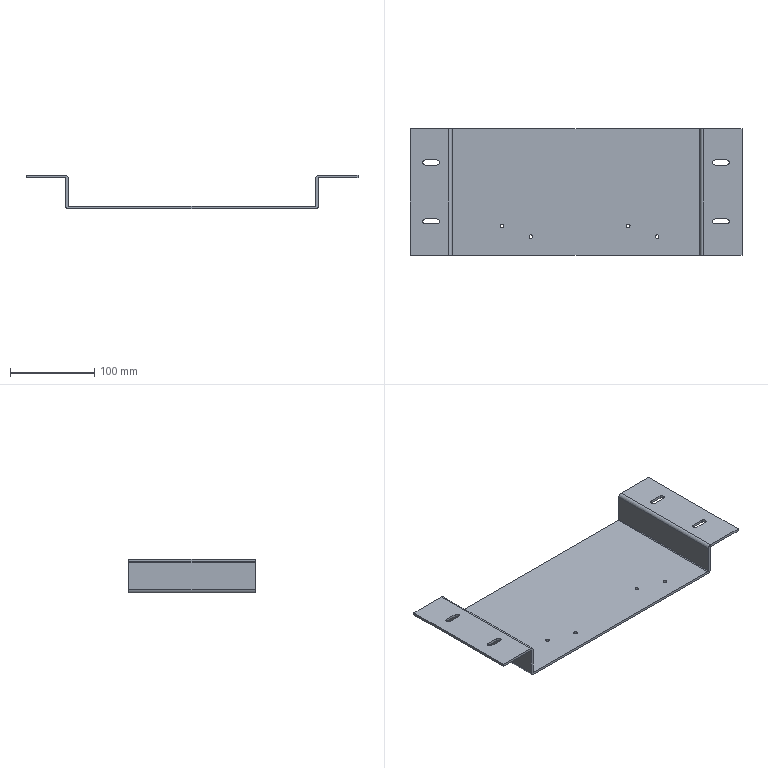Part | SolidWorks | features BaseBody 1 | 1 solid | 46 faces | box 394 x 150 x 40 mm | volume 207359 mm3 | cylinder 24 | plane 22 | commonest cylinder face diameters 4.2 x8 6 x8 1.473 x4 7.473 x4
STEP:
#1=CARTESIAN_POINT('',(98.5,-52.95,0.));
#2=VERTEX_POINT('',#1);
#3=CARTESIAN_POINT('',(94.3,-52.95,0.));
#4=VERTEX_POINT('',#3);
#5=CARTESIAN_POINT('',(96.4,-52.95,0.));
#6=DIRECTION('',(0.,0.,-1.));
#7=DIRECTION('',(-1.,0.,0.));
#8=AXIS2_PLACEMENT_3D('',#5,#6,#7);
#9=CIRCLE('',#8,2.1);
#10=EDGE_CURVE('',#2,#4,#9,.T.);
#11=ORIENTED_EDGE('',*,*,#10,.F.);
#12=CARTESIAN_POINT('',(98.5,-52.95,-3.));
#13=VERTEX_POINT('',#12);
#14=CARTESIAN_POINT('',(98.5,-52.95,-3.));
#15=DIRECTION('',(0.,0.,-1.));
#16=VECTOR('',#15,1000.);
#17=LINE('',#14,#16);
#18=EDGE_CURVE('',#2,#13,#17,.T.);
#19=ORIENTED_EDGE('',*,*,#18,.T.);
#20=CARTESIAN_POINT('',(94.3,-52.95,-3.));
#21=VERTEX_POINT('',#20);
#22=CARTESIAN_POINT('',(96.4,-52.95,-3.));
#23=DIRECTION('',(0.,0.,-1.));
#24=DIRECTION('',(-1.,0.,0.));
#25=AXIS2_PLACEMENT_3D('',#22,#23,#24);
#26=CIRCLE('',#25,2.1);
#27=EDGE_CURVE('',#13,#21,#26,.T.);
#28=ORIENTED_EDGE('',*,*,#27,.T.);
#29=CARTESIAN_POINT('',(94.3,-52.95,-3.));
#30=DIRECTION('',(0.,0.,-1.));
#31=VECTOR('',#30,1000.);
#32=LINE('',#29,#31);
#33=EDGE_CURVE('',#4,#21,#32,.T.);
#34=ORIENTED_EDGE('',*,*,#33,.F.);
#35=EDGE_LOOP('',(#11,#19,#28,#34));
#36=FACE_OUTER_BOUND('',#35,.T.);
#37=CARTESIAN_POINT('',(96.4,-52.95,-3.));
#38=DIRECTION('',(0.,0.,-1.));
#39=DIRECTION('',(-1.,0.,0.));
#40=AXIS2_PLACEMENT_3D('',#37,#38,#39);
#41=CYLINDRICAL_SURFACE('',#40,2.1);
#42=ADVANCED_FACE('',(#36),#41,.F.);
#43=CARTESIAN_POINT('',(64.1,-40.25,0.));
#44=VERTEX_POINT('',#43);
#45=CARTESIAN_POINT('',(59.9,-40.25,0.));
#46=VERTEX_POINT('',#45);
#47=CARTESIAN_POINT('',(62.,-40.25,0.));
#48=DIRECTION('',(0.,0.,-1.));
#49=DIRECTION('',(-1.,0.,0.));
#50=AXIS2_PLACEMENT_3D('',#47,#48,#49);
#51=CIRCLE('',#50,2.1);
#52=EDGE_CURVE('',#44,#46,#51,.T.);
#53=ORIENTED_EDGE('',*,*,#52,.F.);
#54=CARTESIAN_POINT('',(64.1,-40.25,-3.));
#55=VERTEX_POINT('',#54);
#56=CARTESIAN_POINT('',(64.1,-40.25,-3.));
#57=DIRECTION('',(0.,0.,-1.));
#58=VECTOR('',#57,1000.);
#59=LINE('',#56,#58);
#60=EDGE_CURVE('',#44,#55,#59,.T.);
#61=ORIENTED_EDGE('',*,*,#60,.T.);
#62=CARTESIAN_POINT('',(59.9,-40.25,-3.));
#63=VERTEX_POINT('',#62);
#64=CARTESIAN_POINT('',(62.,-40.25,-3.));
#65=DIRECTION('',(0.,0.,-1.));
#66=DIRECTION('',(-1.,0.,0.));
#67=AXIS2_PLACEMENT_3D('',#64,#65,#66);
#68=CIRCLE('',#67,2.1);
#69=EDGE_CURVE('',#55,#63,#68,.T.);
#70=ORIENTED_EDGE('',*,*,#69,.T.);
#71=CARTESIAN_POINT('',(59.9,-40.25,-3.));
#72=DIRECTION('',(0.,0.,-1.));
#73=VECTOR('',#72,1000.);
#74=LINE('',#71,#73);
#75=EDGE_CURVE('',#46,#63,#74,.T.);
#76=ORIENTED_EDGE('',*,*,#75,.F.);
#77=EDGE_LOOP('',(#53,#61,#70,#76));
#78=FACE_OUTER_BOUND('',#77,.T.);
#79=CARTESIAN_POINT('',(62.,-40.25,-3.));
#80=DIRECTION('',(0.,0.,-1.));
#81=DIRECTION('',(-1.,0.,0.));
#82=AXIS2_PLACEMENT_3D('',#79,#80,#81);
#83=CYLINDRICAL_SURFACE('',#82,2.1);
#84=ADVANCED_FACE('',(#78),#83,.F.);
#85=CARTESIAN_POINT('',(-51.5,-52.95,0.));
#86=VERTEX_POINT('',#85);
#87=CARTESIAN_POINT('',(-55.7,-52.95,0.));
#88=VERTEX_POINT('',#87);
#89=CARTESIAN_POINT('',(-53.6,-52.95,0.));
#90=DIRECTION('',(0.,0.,-1.));
#91=DIRECTION('',(-1.,0.,0.));
#92=AXIS2_PLACEMENT_3D('',#89,#90,#91);
#93=CIRCLE('',#92,2.1);
#94=EDGE_CURVE('',#86,#88,#93,.T.);
#95=ORIENTED_EDGE('',*,*,#94,.F.);
#96=CARTESIAN_POINT('',(-51.5,-52.95,-3.));
#97=VERTEX_POINT('',#96);
#98=CARTESIAN_POINT('',(-51.5,-52.95,-3.));
#99=DIRECTION('',(0.,0.,-1.));
#100=VECTOR('',#99,1000.);
#101=LINE('',#98,#100);
#102=EDGE_CURVE('',#86,#97,#101,.T.);
#103=ORIENTED_EDGE('',*,*,#102,.T.);
#104=CARTESIAN_POINT('',(-55.7,-52.95,-3.));
#105=VERTEX_POINT('',#104);
#106=CARTESIAN_POINT('',(-53.6,-52.95,-3.));
#107=DIRECTION('',(0.,0.,-1.));
#108=DIRECTION('',(-1.,0.,0.));
#109=AXIS2_PLACEMENT_3D('',#106,#107,#108);
#110=CIRCLE('',#109,2.1);
#111=EDGE_CURVE('',#97,#105,#110,.T.);
#112=ORIENTED_EDGE('',*,*,#111,.T.);
#113=CARTESIAN_POINT('',(-55.7,-52.95,-3.));
#114=DIRECTION('',(0.,0.,-1.));
#115=VECTOR('',#114,1000.);
#116=LINE('',#113,#115);
#117=EDGE_CURVE('',#88,#105,#116,.T.);
#118=ORIENTED_EDGE('',*,*,#117,.F.);
#119=EDGE_LOOP('',(#95,#103,#112,#118));
#120=FACE_OUTER_BOUND('',#119,.T.);
#121=CARTESIAN_POINT('',(-53.6,-52.95,-3.));
#122=DIRECTION('',(0.,0.,-1.));
#123=DIRECTION('',(-1.,0.,0.));
#124=AXIS2_PLACEMENT_3D('',#121,#122,#123);
#125=CYLINDRICAL_SURFACE('',#124,2.1);
#126=ADVANCED_FACE('',(#120),#125,.F.);
#127=CARTESIAN_POINT('',(-85.9,-40.25,0.));
#128=VERTEX_POINT('',#127);
#129=CARTESIAN_POINT('',(-90.1,-40.25,0.));
#130=VERTEX_POINT('',#129);
#131=CARTESIAN_POINT('',(-88.,-40.25,0.));
#132=DIRECTION('',(0.,0.,-1.));
#133=DIRECTION('',(-1.,0.,0.));
#134=AXIS2_PLACEMENT_3D('',#131,#132,#133);
#135=CIRCLE('',#134,2.1);
#136=EDGE_CURVE('',#128,#130,#135,.T.);
#137=ORIENTED_EDGE('',*,*,#136,.F.);
#138=CARTESIAN_POINT('',(-85.9,-40.25,-3.));
#139=VERTEX_POINT('',#138);
#140=CARTESIAN_POINT('',(-85.9,-40.25,-3.));
#141=DIRECTION('',(0.,0.,-1.));
#142=VECTOR('',#141,1000.);
#143=LINE('',#140,#142);
#144=EDGE_CURVE('',#128,#139,#143,.T.);
#145=ORIENTED_EDGE('',*,*,#144,.T.);
#146=CARTESIAN_POINT('',(-90.1,-40.25,-3.));
#147=VERTEX_POINT('',#146);
#148=CARTESIAN_POINT('',(-88.,-40.25,-3.));
#149=DIRECTION('',(0.,0.,-1.));
#150=DIRECTION('',(-1.,0.,0.));
#151=AXIS2_PLACEMENT_3D('',#148,#149,#150);
#152=CIRCLE('',#151,2.1);
#153=EDGE_CURVE('',#139,#147,#152,.T.);
#154=ORIENTED_EDGE('',*,*,#153,.T.);
#155=CARTESIAN_POINT('',(-90.1,-40.25,-3.));
#156=DIRECTION('',(0.,0.,-1.));
#157=VECTOR('',#156,1000.);
#158=LINE('',#155,#157);
#159=EDGE_CURVE('',#130,#147,#158,.T.);
#160=ORIENTED_EDGE('',*,*,#159,.F.);
#161=EDGE_LOOP('',(#137,#145,#154,#160));
#162=FACE_OUTER_BOUND('',#161,.T.);
#163=CARTESIAN_POINT('',(-88.,-40.25,-3.));
#164=DIRECTION('',(0.,0.,-1.));
#165=DIRECTION('',(-1.,0.,0.));
#166=AXIS2_PLACEMENT_3D('',#163,#164,#165);
#167=CYLINDRICAL_SURFACE('',#166,2.1);
#168=ADVANCED_FACE('',(#162),#167,.F.);
#169=CARTESIAN_POINT('',(165.,32.,34.));
#170=VERTEX_POINT('',#169);
#171=CARTESIAN_POINT('',(165.,32.,37.));
#172=VERTEX_POINT('',#171);
#173=CARTESIAN_POINT('',(165.,32.,34.));
#174=DIRECTION('',(0.,0.,1.));
#175=VECTOR('',#174,1000.);
#176=LINE('',#173,#175);
#177=EDGE_CURVE('',#170,#172,#176,.T.);
#178=ORIENTED_EDGE('',*,*,#177,.T.);
#179=CARTESIAN_POINT('',(179.,32.,37.));
#180=VERTEX_POINT('',#179);
#181=CARTESIAN_POINT('',(179.,32.,37.));
#182=DIRECTION('',(-1.,0.,0.));
#183=VECTOR('',#182,1000.);
#184=LINE('',#181,#183);
#185=EDGE_CURVE('',#180,#172,#184,.T.);
#186=ORIENTED_EDGE('',*,*,#185,.F.);
#187=CARTESIAN_POINT('',(179.,32.,34.));
#188=VERTEX_POINT('',#187);
#189=CARTESIAN_POINT('',(179.,32.,34.));
#190=DIRECTION('',(0.,0.,-1.));
#191=VECTOR('',#190,1000.);
#192=LINE('',#189,#191);
#193=EDGE_CURVE('',#180,#188,#192,.T.);
#194=ORIENTED_EDGE('',*,*,#193,.T.);
#195=CARTESIAN_POINT('',(179.,32.,34.));
#196=DIRECTION('',(-1.,0.,0.));
#197=VECTOR('',#196,1000.);
#198=LINE('',#195,#197);
#199=EDGE_CURVE('',#188,#170,#198,.T.);
#200=ORIENTED_EDGE('',*,*,#199,.T.);
#201=EDGE_LOOP('',(#178,#186,#194,#200));
#202=FACE_OUTER_BOUND('',#201,.T.);
#203=CARTESIAN_POINT('',(179.,32.,34.));
#204=DIRECTION('',(0.,-1.,0.));
#205=DIRECTION('',(-1.,0.,0.));
#206=AXIS2_PLACEMENT_3D('',#203,#204,#205);
#207=PLANE('',#206);
#208=ADVANCED_FACE('',(#202),#207,.F.);
#209=CARTESIAN_POINT('',(165.,38.,37.));
#210=VERTEX_POINT('',#209);
#211=CARTESIAN_POINT('',(165.,38.,34.));
#212=VERTEX_POINT('',#211);
#213=CARTESIAN_POINT('',(165.,38.,34.));
#214=DIRECTION('',(0.,0.,-1.));
#215=VECTOR('',#214,1000.);
#216=LINE('',#213,#215);
#217=EDGE_CURVE('',#210,#212,#216,.T.);
#218=ORIENTED_EDGE('',*,*,#217,.T.);
#219=CARTESIAN_POINT('',(179.,38.,34.));
#220=VERTEX_POINT('',#219);
#221=CARTESIAN_POINT('',(179.,38.,34.));
#222=DIRECTION('',(-1.,0.,0.));
#223=VECTOR('',#222,1000.);
#224=LINE('',#221,#223);
#225=EDGE_CURVE('',#220,#212,#224,.T.);
#226=ORIENTED_EDGE('',*,*,#225,.F.);
#227=CARTESIAN_POINT('',(179.,38.,37.));
#228=VERTEX_POINT('',#227);
#229=CARTESIAN_POINT('',(179.,38.,34.));
#230=DIRECTION('',(0.,0.,1.));
#231=VECTOR('',#230,1000.);
#232=LINE('',#229,#231);
#233=EDGE_CURVE('',#220,#228,#232,.T.);
#234=ORIENTED_EDGE('',*,*,#233,.T.);
#235=CARTESIAN_POINT('',(179.,38.,37.));
#236=DIRECTION('',(-1.,0.,0.));
#237=VECTOR('',#236,1000.);
#238=LINE('',#235,#237);
#239=EDGE_CURVE('',#228,#210,#238,.T.);
#240=ORIENTED_EDGE('',*,*,#239,.T.);
#241=EDGE_LOOP('',(#218,#226,#234,#240));
#242=FACE_OUTER_BOUND('',#241,.T.);
#243=CARTESIAN_POINT('',(179.,38.,34.));
#244=DIRECTION('',(0.,1.,0.));
#245=DIRECTION('',(0.,0.,-1.));
#246=AXIS2_PLACEMENT_3D('',#243,#244,#245);
#247=PLANE('',#246);
#248=ADVANCED_FACE('',(#242),#247,.F.);
#249=CARTESIAN_POINT('',(179.,35.,34.));
#250=DIRECTION('',(0.,0.,-1.));
#251=DIRECTION('',(0.,1.,0.));
#252=AXIS2_PLACEMENT_3D('',#249,#250,#251);
#253=CIRCLE('',#252,3.);
#254=EDGE_CURVE('',#220,#188,#253,.T.);
#255=ORIENTED_EDGE('',*,*,#254,.T.);
#256=ORIENTED_EDGE('',*,*,#193,.F.);
#257=CARTESIAN_POINT('',(179.,35.,37.));
#258=DIRECTION('',(0.,0.,-1.));
#259=DIRECTION('',(0.,1.,0.));
#260=AXIS2_PLACEMENT_3D('',#257,#258,#259);
#261=CIRCLE('',#260,3.);
#262=EDGE_CURVE('',#228,#180,#261,.T.);
#263=ORIENTED_EDGE('',*,*,#262,.F.);
#264=ORIENTED_EDGE('',*,*,#233,.F.);
#265=EDGE_LOOP('',(#255,#256,#263,#264));
#266=FACE_OUTER_BOUND('',#265,.T.);
#267=CARTESIAN_POINT('',(179.,35.,34.));
#268=DIRECTION('',(0.,0.,-1.));
#269=DIRECTION('',(0.,1.,0.));
#270=AXIS2_PLACEMENT_3D('',#267,#268,#269);
#271=CYLINDRICAL_SURFACE('',#270,3.);
#272=ADVANCED_FACE('',(#266),#271,.F.);
#273=CARTESIAN_POINT('',(165.,35.,34.));
#274=DIRECTION('',(0.,0.,-1.));
#275=DIRECTION('',(0.,1.,0.));
#276=AXIS2_PLACEMENT_3D('',#273,#274,#275);
#277=CIRCLE('',#276,3.);
#278=EDGE_CURVE('',#170,#212,#277,.T.);
#279=ORIENTED_EDGE('',*,*,#278,.T.);
#280=ORIENTED_EDGE('',*,*,#217,.F.);
#281=CARTESIAN_POINT('',(165.,35.,37.));
#282=DIRECTION('',(0.,0.,-1.));
#283=DIRECTION('',(0.,1.,0.));
#284=AXIS2_PLACEMENT_3D('',#281,#282,#283);
#285=CIRCLE('',#284,3.);
#286=EDGE_CURVE('',#172,#210,#285,.T.);
#287=ORIENTED_EDGE('',*,*,#286,.F.);
#288=ORIENTED_EDGE('',*,*,#177,.F.);
#289=EDGE_LOOP('',(#279,#280,#287,#288));
#290=FACE_OUTER_BOUND('',#289,.T.);
#291=CARTESIAN_POINT('',(165.,35.,34.));
#292=DIRECTION('',(0.,0.,-1.));
#293=DIRECTION('',(0.,1.,0.));
#294=AXIS2_PLACEMENT_3D('',#291,#292,#293);
#295=CYLINDRICAL_SURFACE('',#294,3.);
#296=ADVANCED_FACE('',(#290),#295,.F.);
#297=CARTESIAN_POINT('',(165.,-38.,34.));
#298=VERTEX_POINT('',#297);
#299=CARTESIAN_POINT('',(165.,-38.,37.));
#300=VERTEX_POINT('',#299);
#301=CARTESIAN_POINT('',(165.,-38.,34.));
#302=DIRECTION('',(0.,0.,1.));
#303=VECTOR('',#302,1000.);
#304=LINE('',#301,#303);
#305=EDGE_CURVE('',#298,#300,#304,.T.);
#306=ORIENTED_EDGE('',*,*,#305,.T.);
#307=CARTESIAN_POINT('',(179.,-38.,37.));
#308=VERTEX_POINT('',#307);
#309=CARTESIAN_POINT('',(179.,-38.,37.));
#310=DIRECTION('',(-1.,0.,0.));
#311=VECTOR('',#310,1000.);
#312=LINE('',#309,#311);
#313=EDGE_CURVE('',#308,#300,#312,.T.);
#314=ORIENTED_EDGE('',*,*,#313,.F.);
#315=CARTESIAN_POINT('',(179.,-38.,34.));
#316=VERTEX_POINT('',#315);
#317=CARTESIAN_POINT('',(179.,-38.,34.));
#318=DIRECTION('',(0.,0.,-1.));
#319=VECTOR('',#318,1000.);
#320=LINE('',#317,#319);
#321=EDGE_CURVE('',#308,#316,#320,.T.);
#322=ORIENTED_EDGE('',*,*,#321,.T.);
#323=CARTESIAN_POINT('',(179.,-38.,34.));
#324=DIRECTION('',(-1.,0.,0.));
#325=VECTOR('',#324,1000.);
#326=LINE('',#323,#325);
#327=EDGE_CURVE('',#316,#298,#326,.T.);
#328=ORIENTED_EDGE('',*,*,#327,.T.);
#329=EDGE_LOOP('',(#306,#314,#322,#328));
#330=FACE_OUTER_BOUND('',#329,.T.);
#331=CARTESIAN_POINT('',(179.,-38.,34.));
#332=DIRECTION('',(0.,-1.,0.));
#333=DIRECTION('',(-1.,0.,0.));
#334=AXIS2_PLACEMENT_3D('',#331,#332,#333);
#335=PLANE('',#334);
#336=ADVANCED_FACE('',(#330),#335,.F.);
#337=CARTESIAN_POINT('',(165.,-32.,37.));
#338=VERTEX_POINT('',#337);
#339=CARTESIAN_POINT('',(165.,-32.,34.));
#340=VERTEX_POINT('',#339);
#341=CARTESIAN_POINT('',(165.,-32.,34.));
#342=DIRECTION('',(0.,0.,-1.));
#343=VECTOR('',#342,1000.);
#344=LINE('',#341,#343);
#345=EDGE_CURVE('',#338,#340,#344,.T.);
#346=ORIENTED_EDGE('',*,*,#345,.T.);
#347=CARTESIAN_POINT('',(179.,-32.,34.));
#348=VERTEX_POINT('',#347);
#349=CARTESIAN_POINT('',(179.,-32.,34.));
#350=DIRECTION('',(-1.,0.,0.));
#351=VECTOR('',#350,1000.);
#352=LINE('',#349,#351);
#353=EDGE_CURVE('',#348,#340,#352,.T.);
#354=ORIENTED_EDGE('',*,*,#353,.F.);
#355=CARTESIAN_POINT('',(179.,-32.,37.));
#356=VERTEX_POINT('',#355);
#357=CARTESIAN_POINT('',(179.,-32.,34.));
#358=DIRECTION('',(0.,0.,1.));
#359=VECTOR('',#358,1000.);
#360=LINE('',#357,#359);
#361=EDGE_CURVE('',#348,#356,#360,.T.);
#362=ORIENTED_EDGE('',*,*,#361,.T.);
#363=CARTESIAN_POINT('',(179.,-32.,37.));
#364=DIRECTION('',(-1.,0.,0.));
#365=VECTOR('',#364,1000.);
#366=LINE('',#363,#365);
#367=EDGE_CURVE('',#356,#338,#366,.T.);
#368=ORIENTED_EDGE('',*,*,#367,.T.);
#369=EDGE_LOOP('',(#346,#354,#362,#368));
#370=FACE_OUTER_BOUND('',#369,.T.);
#371=CARTESIAN_POINT('',(179.,-32.,34.));
#372=DIRECTION('',(0.,1.,0.));
#373=DIRECTION('',(0.,0.,-1.));
#374=AXIS2_PLACEMENT_3D('',#371,#372,#373);
#375=PLANE('',#374);
#376=ADVANCED_FACE('',(#370),#375,.F.);
#377=CARTESIAN_POINT('',(179.,-35.,34.));
#378=DIRECTION('',(0.,0.,-1.));
#379=DIRECTION('',(0.,1.,0.));
#380=AXIS2_PLACEMENT_3D('',#377,#378,#379);
#381=CIRCLE('',#380,3.);
#382=EDGE_CURVE('',#348,#316,#381,.T.);
#383=ORIENTED_EDGE('',*,*,#382,.T.);
#384=ORIENTED_EDGE('',*,*,#321,.F.);
#385=CARTESIAN_POINT('',(179.,-35.,37.));
#386=DIRECTION('',(0.,0.,-1.));
#387=DIRECTION('',(0.,1.,0.));
#388=AXIS2_PLACEMENT_3D('',#385,#386,#387);
#389=CIRCLE('',#388,3.);
#390=EDGE_CURVE('',#356,#308,#389,.T.);
#391=ORIENTED_EDGE('',*,*,#390,.F.);
#392=ORIENTED_EDGE('',*,*,#361,.F.);
#393=EDGE_LOOP('',(#383,#384,#391,#392));
#394=FACE_OUTER_BOUND('',#393,.T.);
#395=CARTESIAN_POINT('',(179.,-35.,34.));
#396=DIRECTION('',(0.,0.,-1.));
#397=DIRECTION('',(0.,1.,0.));
#398=AXIS2_PLACEMENT_3D('',#395,#396,#397);
#399=CYLINDRICAL_SURFACE('',#398,3.);
#400=ADVANCED_FACE('',(#394),#399,.F.);
#401=CARTESIAN_POINT('',(165.,-35.,34.));
#402=DIRECTION('',(0.,0.,-1.));
#403=DIRECTION('',(0.,1.,0.));
#404=AXIS2_PLACEMENT_3D('',#401,#402,#403);
#405=CIRCLE('',#404,3.);
#406=EDGE_CURVE('',#298,#340,#405,.T.);
#407=ORIENTED_EDGE('',*,*,#406,.T.);
#408=ORIENTED_EDGE('',*,*,#345,.F.);
#409=CARTESIAN_POINT('',(165.,-35.,37.));
#410=DIRECTION('',(0.,0.,-1.));
#411=DIRECTION('',(0.,1.,0.));
#412=AXIS2_PLACEMENT_3D('',#409,#410,#411);
#413=CIRCLE('',#412,3.);
#414=EDGE_CURVE('',#300,#338,#413,.T.);
#415=ORIENTED_EDGE('',*,*,#414,.F.);
#416=ORIENTED_EDGE('',*,*,#305,.F.);
#417=EDGE_LOOP('',(#407,#408,#415,#416));
#418=FACE_OUTER_BOUND('',#417,.T.);
#419=CARTESIAN_POINT('',(165.,-35.,34.));
#420=DIRECTION('',(0.,0.,-1.));
#421=DIRECTION('',(0.,1.,0.));
#422=AXIS2_PLACEMENT_3D('',#419,#420,#421);
#423=CYLINDRICAL_SURFACE('',#422,3.);
#424=ADVANCED_FACE('',(#418),#423,.F.);
#425=CARTESIAN_POINT('',(-179.,-38.,34.));
#426=VERTEX_POINT('',#425);
#427=CARTESIAN_POINT('',(-179.,-38.,37.));
#428=VERTEX_POINT('',#427);
#429=CARTESIAN_POINT('',(-179.,-38.,34.));
#430=DIRECTION('',(0.,0.,1.));
#431=VECTOR('',#430,1000.);
#432=LINE('',#429,#431);
#433=EDGE_CURVE('',#426,#428,#432,.T.);
#434=ORIENTED_EDGE('',*,*,#433,.T.);
#435=CARTESIAN_POINT('',(-165.,-38.,37.));
#436=VERTEX_POINT('',#435);
#437=CARTESIAN_POINT('',(-165.,-38.,37.));
#438=DIRECTION('',(-1.,0.,0.));
#439=VECTOR('',#438,1000.);
#440=LINE('',#437,#439);
#441=EDGE_CURVE('',#436,#428,#440,.T.);
#442=ORIENTED_EDGE('',*,*,#441,.F.);
#443=CARTESIAN_POINT('',(-165.,-38.,34.));
#444=VERTEX_POINT('',#443);
#445=CARTESIAN_POINT('',(-165.,-38.,34.));
#446=DIRECTION('',(0.,0.,-1.));
#447=VECTOR('',#446,1000.);
#448=LINE('',#445,#447);
#449=EDGE_CURVE('',#436,#444,#448,.T.);
#450=ORIENTED_EDGE('',*,*,#449,.T.);
#451=CARTESIAN_POINT('',(-165.,-38.,34.));
#452=DIRECTION('',(-1.,0.,0.));
#453=VECTOR('',#452,1000.);
#454=LINE('',#451,#453);
#455=EDGE_CURVE('',#444,#426,#454,.T.);
#456=ORIENTED_EDGE('',*,*,#455,.T.);
#457=EDGE_LOOP('',(#434,#442,#450,#456));
#458=FACE_OUTER_BOUND('',#457,.T.);
#459=CARTESIAN_POINT('',(-165.,-38.,34.));
#460=DIRECTION('',(0.,-1.,0.));
#461=DIRECTION('',(-1.,0.,0.));
#462=AXIS2_PLACEMENT_3D('',#459,#460,#461);
#463=PLANE('',#462);
#464=ADVANCED_FACE('',(#458),#463,.F.);
#465=CARTESIAN_POINT('',(-179.,-32.,37.));
#466=VERTEX_POINT('',#465);
#467=CARTESIAN_POINT('',(-179.,-32.,34.));
#468=VERTEX_POINT('',#467);
#469=CARTESIAN_POINT('',(-179.,-32.,34.));
#470=DIRECTION('',(0.,0.,-1.));
#471=VECTOR('',#470,1000.);
#472=LINE('',#469,#471);
#473=EDGE_CURVE('',#466,#468,#472,.T.);
#474=ORIENTED_EDGE('',*,*,#473,.T.);
#475=CARTESIAN_POINT('',(-165.,-32.,34.));
#476=VERTEX_POINT('',#475);
#477=CARTESIAN_POINT('',(-165.,-32.,34.));
#478=DIRECTION('',(-1.,0.,0.));
#479=VECTOR('',#478,1000.);
#480=LINE('',#477,#479);
#481=EDGE_CURVE('',#476,#468,#480,.T.);
#482=ORIENTED_EDGE('',*,*,#481,.F.);
#483=CARTESIAN_POINT('',(-165.,-32.,37.));
#484=VERTEX_POINT('',#483);
#485=CARTESIAN_POINT('',(-165.,-32.,34.));
#486=DIRECTION('',(0.,0.,1.));
#487=VECTOR('',#486,1000.);
#488=LINE('',#485,#487);
#489=EDGE_CURVE('',#476,#484,#488,.T.);
#490=ORIENTED_EDGE('',*,*,#489,.T.);
#491=CARTESIAN_POINT('',(-165.,-32.,37.));
#492=DIRECTION('',(-1.,0.,0.));
#493=VECTOR('',#492,1000.);
#494=LINE('',#491,#493);
#495=EDGE_CURVE('',#484,#466,#494,.T.);
#496=ORIENTED_EDGE('',*,*,#495,.T.);
#497=EDGE_LOOP('',(#474,#482,#490,#496));
#498=FACE_OUTER_BOUND('',#497,.T.);
#499=CARTESIAN_POINT('',(-165.,-32.,34.));
#500=DIRECTION('',(0.,1.,0.));
#501=DIRECTION('',(0.,0.,-1.));
#502=AXIS2_PLACEMENT_3D('',#499,#500,#501);
#503=PLANE('',#502);
#504=ADVANCED_FACE('',(#498),#503,.F.);
#505=CARTESIAN_POINT('',(-165.,-35.,34.));
#506=DIRECTION('',(0.,0.,-1.));
#507=DIRECTION('',(0.,1.,0.));
#508=AXIS2_PLACEMENT_3D('',#505,#506,#507);
#509=CIRCLE('',#508,3.);
#510=EDGE_CURVE('',#476,#444,#509,.T.);
#511=ORIENTED_EDGE('',*,*,#510,.T.);
#512=ORIENTED_EDGE('',*,*,#449,.F.);
#513=CARTESIAN_POINT('',(-165.,-35.,37.));
#514=DIRECTION('',(0.,0.,-1.));
#515=DIRECTION('',(0.,1.,0.));
#516=AXIS2_PLACEMENT_3D('',#513,#514,#515);
#517=CIRCLE('',#516,3.);
#518=EDGE_CURVE('',#484,#436,#517,.T.);
#519=ORIENTED_EDGE('',*,*,#518,.F.);
#520=ORIENTED_EDGE('',*,*,#489,.F.);
#521=EDGE_LOOP('',(#511,#512,#519,#520));
#522=FACE_OUTER_BOUND('',#521,.T.);
#523=CARTESIAN_POINT('',(-165.,-35.,34.));
#524=DIRECTION('',(0.,0.,-1.));
#525=DIRECTION('',(0.,1.,0.));
#526=AXIS2_PLACEMENT_3D('',#523,#524,#525);
#527=CYLINDRICAL_SURFACE('',#526,3.);
#528=ADVANCED_FACE('',(#522),#527,.F.);
#529=CARTESIAN_POINT('',(-179.,-35.,34.));
#530=DIRECTION('',(0.,0.,-1.));
#531=DIRECTION('',(0.,1.,0.));
#532=AXIS2_PLACEMENT_3D('',#529,#530,#531);
#533=CIRCLE('',#532,3.);
#534=EDGE_CURVE('',#426,#468,#533,.T.);
#535=ORIENTED_EDGE('',*,*,#534,.T.);
#536=ORIENTED_EDGE('',*,*,#473,.F.);
#537=CARTESIAN_POINT('',(-179.,-35.,37.));
#538=DIRECTION('',(0.,0.,-1.));
#539=DIRECTION('',(0.,1.,0.));
#540=AXIS2_PLACEMENT_3D('',#537,#538,#539);
#541=CIRCLE('',#540,3.);
#542=EDGE_CURVE('',#428,#466,#541,.T.);
#543=ORIENTED_EDGE('',*,*,#542,.F.);
#544=ORIENTED_EDGE('',*,*,#433,.F.);
#545=EDGE_LOOP('',(#535,#536,#543,#544));
#546=FACE_OUTER_BOUND('',#545,.T.);
#547=CARTESIAN_POINT('',(-179.,-35.,34.));
#548=DIRECTION('',(0.,0.,-1.));
#549=DIRECTION('',(0.,1.,0.));
#550=AXIS2_PLACEMENT_3D('',#547,#548,#549);
#551=CYLINDRICAL_SURFACE('',#550,3.);
#552=ADVANCED_FACE('',(#546),#551,.F.);
#553=CARTESIAN_POINT('',(-179.,32.,34.));
#554=VERTEX_POINT('',#553);
#555=CARTESIAN_POINT('',(-179.,32.,37.));
#556=VERTEX_POINT('',#555);
#557=CARTESIAN_POINT('',(-179.,32.,34.));
#558=DIRECTION('',(0.,0.,1.));
#559=VECTOR('',#558,1000.);
#560=LINE('',#557,#559);
#561=EDGE_CURVE('',#554,#556,#560,.T.);
#562=ORIENTED_EDGE('',*,*,#561,.T.);
#563=CARTESIAN_POINT('',(-165.,32.,37.));
#564=VERTEX_POINT('',#563);
#565=CARTESIAN_POINT('',(-165.,32.,37.));
#566=DIRECTION('',(-1.,0.,0.));
#567=VECTOR('',#566,1000.);
#568=LINE('',#565,#567);
#569=EDGE_CURVE('',#564,#556,#568,.T.);
#570=ORIENTED_EDGE('',*,*,#569,.F.);
#571=CARTESIAN_POINT('',(-165.,32.,34.));
#572=VERTEX_POINT('',#571);
#573=CARTESIAN_POINT('',(-165.,32.,34.));
#574=DIRECTION('',(0.,0.,-1.));
#575=VECTOR('',#574,1000.);
#576=LINE('',#573,#575);
#577=EDGE_CURVE('',#564,#572,#576,.T.);
#578=ORIENTED_EDGE('',*,*,#577,.T.);
#579=CARTESIAN_POINT('',(-165.,32.,34.));
#580=DIRECTION('',(-1.,0.,0.));
#581=VECTOR('',#580,1000.);
#582=LINE('',#579,#581);
#583=EDGE_CURVE('',#572,#554,#582,.T.);
#584=ORIENTED_EDGE('',*,*,#583,.T.);
#585=EDGE_LOOP('',(#562,#570,#578,#584));
#586=FACE_OUTER_BOUND('',#585,.T.);
#587=CARTESIAN_POINT('',(-165.,32.,34.));
#588=DIRECTION('',(0.,-1.,0.));
#589=DIRECTION('',(-1.,0.,0.));
#590=AXIS2_PLACEMENT_3D('',#587,#588,#589);
#591=PLANE('',#590);
#592=ADVANCED_FACE('',(#586),#591,.F.);
#593=CARTESIAN_POINT('',(-179.,38.,37.));
#594=VERTEX_POINT('',#593);
#595=CARTESIAN_POINT('',(-179.,38.,34.));
#596=VERTEX_POINT('',#595);
#597=CARTESIAN_POINT('',(-179.,38.,34.));
#598=DIRECTION('',(0.,0.,-1.));
#599=VECTOR('',#598,1000.);
#600=LINE('',#597,#599);
#601=EDGE_CURVE('',#594,#596,#600,.T.);
#602=ORIENTED_EDGE('',*,*,#601,.T.);
#603=CARTESIAN_POINT('',(-165.,38.,34.));
#604=VERTEX_POINT('',#603);
#605=CARTESIAN_POINT('',(-165.,38.,34.));
#606=DIRECTION('',(-1.,0.,0.));
#607=VECTOR('',#606,1000.);
#608=LINE('',#605,#607);
#609=EDGE_CURVE('',#604,#596,#608,.T.);
#610=ORIENTED_EDGE('',*,*,#609,.F.);
#611=CARTESIAN_POINT('',(-165.,38.,37.));
#612=VERTEX_POINT('',#611);
#613=CARTESIAN_POINT('',(-165.,38.,34.));
#614=DIRECTION('',(0.,0.,1.));
#615=VECTOR('',#614,1000.);
#616=LINE('',#613,#615);
#617=EDGE_CURVE('',#604,#612,#616,.T.);
#618=ORIENTED_EDGE('',*,*,#617,.T.);
#619=CARTESIAN_POINT('',(-165.,38.,37.));
#620=DIRECTION('',(-1.,0.,0.));
#621=VECTOR('',#620,1000.);
#622=LINE('',#619,#621);
#623=EDGE_CURVE('',#612,#594,#622,.T.);
#624=ORIENTED_EDGE('',*,*,#623,.T.);
#625=EDGE_LOOP('',(#602,#610,#618,#624));
#626=FACE_OUTER_BOUND('',#625,.T.);
#627=CARTESIAN_POINT('',(-165.,38.,34.));
#628=DIRECTION('',(0.,1.,0.));
#629=DIRECTION('',(0.,0.,-1.));
#630=AXIS2_PLACEMENT_3D('',#627,#628,#629);
#631=PLANE('',#630);
#632=ADVANCED_FACE('',(#626),#631,.F.);
#633=CARTESIAN_POINT('',(-165.,35.,34.));
#634=DIRECTION('',(0.,0.,-1.));
#635=DIRECTION('',(0.,1.,0.));
#636=AXIS2_PLACEMENT_3D('',#633,#634,#635);
#637=CIRCLE('',#636,3.);
#638=EDGE_CURVE('',#604,#572,#637,.T.);
#639=ORIENTED_EDGE('',*,*,#638,.T.);
#640=ORIENTED_EDGE('',*,*,#577,.F.);
#641=CARTESIAN_POINT('',(-165.,35.,37.));
#642=DIRECTION('',(0.,0.,-1.));
#643=DIRECTION('',(0.,1.,0.));
#644=AXIS2_PLACEMENT_3D('',#641,#642,#643);
#645=CIRCLE('',#644,3.);
#646=EDGE_CURVE('',#612,#564,#645,.T.);
#647=ORIENTED_EDGE('',*,*,#646,.F.);
#648=ORIENTED_EDGE('',*,*,#617,.F.);
#649=EDGE_LOOP('',(#639,#640,#647,#648));
#650=FACE_OUTER_BOUND('',#649,.T.);
#651=CARTESIAN_POINT('',(-165.,35.,34.));
#652=DIRECTION('',(0.,0.,-1.));
#653=DIRECTION('',(0.,1.,0.));
#654=AXIS2_PLACEMENT_3D('',#651,#652,#653);
#655=CYLINDRICAL_SURFACE('',#654,3.);
#656=ADVANCED_FACE('',(#650),#655,.F.);
#657=CARTESIAN_POINT('',(-179.,35.,34.));
#658=DIRECTION('',(0.,0.,-1.));
#659=DIRECTION('',(0.,1.,0.));
#660=AXIS2_PLACEMENT_3D('',#657,#658,#659);
#661=CIRCLE('',#660,3.);
#662=EDGE_CURVE('',#554,#596,#661,.T.);
#663=ORIENTED_EDGE('',*,*,#662,.T.);
#664=ORIENTED_EDGE('',*,*,#601,.F.);
#665=CARTESIAN_POINT('',(-179.,35.,37.));
#666=DIRECTION('',(0.,0.,-1.));
#667=DIRECTION('',(0.,1.,0.));
#668=AXIS2_PLACEMENT_3D('',#665,#666,#667);
#669=CIRCLE('',#668,3.);
#670=EDGE_CURVE('',#556,#594,#669,.T.);
#671=ORIENTED_EDGE('',*,*,#670,.F.);
#672=ORIENTED_EDGE('',*,*,#561,.F.);
#673=EDGE_LOOP('',(#663,#664,#671,#672));
#674=FACE_OUTER_BOUND('',#673,.T.);
#675=CARTESIAN_POINT('',(-179.,35.,34.));
#676=DIRECTION('',(0.,0.,-1.));
#677=DIRECTION('',(0.,1.,0.));
#678=AXIS2_PLACEMENT_3D('',#675,#676,#677);
#679=CYLINDRICAL_SURFACE('',#678,3.);
#680=ADVANCED_FACE('',(#674),#679,.F.);
#681=CARTESIAN_POINT('',(197.,75.,34.));
#682=VERTEX_POINT('',#681);
#683=CARTESIAN_POINT('',(197.,-75.,34.));
#684=VERTEX_POINT('',#683);
#685=CARTESIAN_POINT('',(197.,0.,34.));
#686=DIRECTION('',(0.,-1.,0.));
#687=VECTOR('',#686,1000.);
#688=LINE('',#685,#687);
#689=EDGE_CURVE('',#682,#684,#688,.T.);
#690=ORIENTED_EDGE('',*,*,#689,.F.);
#691=CARTESIAN_POINT('',(197.,75.,37.));
#692=VERTEX_POINT('',#691);
#693=CARTESIAN_POINT('',(197.,75.,37.));
#694=DIRECTION('',(0.,0.,-1.));
#695=VECTOR('',#694,1000.);
#696=LINE('',#693,#695);
#697=EDGE_CURVE('',#692,#682,#696,.T.);
#698=ORIENTED_EDGE('',*,*,#697,.F.);
#699=CARTESIAN_POINT('',(197.,-75.,37.));
#700=VERTEX_POINT('',#699);
#701=CARTESIAN_POINT('',(197.,75.,37.));
#702=DIRECTION('',(0.,-1.,0.));
#703=VECTOR('',#702,1000.);
#704=LINE('',#701,#703);
#705=EDGE_CURVE('',#692,#700,#704,.T.);
#706=ORIENTED_EDGE('',*,*,#705,.T.);
#707=CARTESIAN_POINT('',(197.,-75.,37.));
#708=DIRECTION('',(0.,0.,-1.));
#709=VECTOR('',#708,1000.);
#710=LINE('',#707,#709);
#711=EDGE_CURVE('',#700,#684,#710,.T.);
#712=ORIENTED_EDGE('',*,*,#711,.T.);
#713=EDGE_LOOP('',(#690,#698,#706,#712));
#714=FACE_OUTER_BOUND('',#713,.T.);
#715=CARTESIAN_POINT('',(197.,75.,37.));
#716=DIRECTION('',(1.,0.,0.));
#717=DIRECTION('',(0.,0.,-1.));
#718=AXIS2_PLACEMENT_3D('',#715,#716,#717);
#719=PLANE('',#718);
#720=ADVANCED_FACE('',(#714),#719,.T.);
#721=ORIENTED_EDGE('',*,*,#327,.F.);
#722=ORIENTED_EDGE('',*,*,#382,.F.);
#723=ORIENTED_EDGE('',*,*,#353,.T.);
#724=ORIENTED_EDGE('',*,*,#406,.F.);
#725=EDGE_LOOP('',(#721,#722,#723,#724));
#726=FACE_BOUND('',#725,.T.);
#727=ORIENTED_EDGE('',*,*,#225,.T.);
#728=ORIENTED_EDGE('',*,*,#278,.F.);
#729=ORIENTED_EDGE('',*,*,#199,.F.);
#730=ORIENTED_EDGE('',*,*,#254,.F.);
#731=EDGE_LOOP('',(#727,#728,#729,#730));
#732=FACE_BOUND('',#731,.T.);
#733=CARTESIAN_POINT('',(150.737,-75.,34.));
#734=VERTEX_POINT('',#733);
#735=CARTESIAN_POINT('',(0.,-75.,34.));
#736=DIRECTION('',(-1.,0.,0.));
#737=VECTOR('',#736,1000.);
#738=LINE('',#735,#737);
#739=EDGE_CURVE('',#684,#734,#738,.T.);
#740=ORIENTED_EDGE('',*,*,#739,.T.);
#741=CARTESIAN_POINT('',(150.737,75.,34.));
#742=VERTEX_POINT('',#741);
#743=CARTESIAN_POINT('',(150.737,75.,34.));
#744=DIRECTION('',(0.,-1.,0.));
#745=VECTOR('',#744,1000.);
#746=LINE('',#743,#745);
#747=EDGE_CURVE('',#742,#734,#746,.T.);
#748=ORIENTED_EDGE('',*,*,#747,.F.);
#749=CARTESIAN_POINT('',(0.,75.,34.));
#750=DIRECTION('',(1.,0.,0.));
#751=VECTOR('',#750,1000.);
#752=LINE('',#749,#751);
#753=EDGE_CURVE('',#742,#682,#752,.T.);
#754=ORIENTED_EDGE('',*,*,#753,.T.);
#755=ORIENTED_EDGE('',*,*,#689,.T.);
#756=EDGE_LOOP('',(#740,#748,#754,#755));
#757=FACE_OUTER_BOUND('',#756,.T.);
#758=CARTESIAN_POINT('',(0.,0.,34.));
#759=DIRECTION('',(0.,0.,-1.));
#760=DIRECTION('',(-1.,0.,0.));
#761=AXIS2_PLACEMENT_3D('',#758,#759,#760);
#762=PLANE('',#761);
#763=ADVANCED_FACE('',(#726,#732,#757),#762,.T.);
#764=ORIENTED_EDGE('',*,*,#390,.T.);
#765=ORIENTED_EDGE('',*,*,#313,.T.);
#766=ORIENTED_EDGE('',*,*,#414,.T.);
#767=ORIENTED_EDGE('',*,*,#367,.F.);
#768=EDGE_LOOP('',(#764,#765,#766,#767));
#769=FACE_BOUND('',#768,.T.);
#770=ORIENTED_EDGE('',*,*,#262,.T.);
#771=ORIENTED_EDGE('',*,*,#185,.T.);
#772=ORIENTED_EDGE('',*,*,#286,.T.);
#773=ORIENTED_EDGE('',*,*,#239,.F.);
#774=EDGE_LOOP('',(#770,#771,#772,#773));
#775=FACE_BOUND('',#774,.T.);
#776=CARTESIAN_POINT('',(150.737,-75.,37.));
#777=VERTEX_POINT('',#776);
#778=CARTESIAN_POINT('',(150.737,75.,37.));
#779=VERTEX_POINT('',#778);
#780=CARTESIAN_POINT('',(150.737,75.,37.));
#781=DIRECTION('',(0.,1.,0.));
#782=VECTOR('',#781,1000.);
#783=LINE('',#780,#782);
#784=EDGE_CURVE('',#777,#779,#783,.T.);
#785=ORIENTED_EDGE('',*,*,#784,.F.);
#786=CARTESIAN_POINT('',(197.,-75.,37.));
#787=DIRECTION('',(-1.,0.,0.));
#788=VECTOR('',#787,1000.);
#789=LINE('',#786,#788);
#790=EDGE_CURVE('',#700,#777,#789,.T.);
#791=ORIENTED_EDGE('',*,*,#790,.F.);
#792=ORIENTED_EDGE('',*,*,#705,.F.);
#793=CARTESIAN_POINT('',(150.,75.,37.));
#794=DIRECTION('',(1.,0.,0.));
#795=VECTOR('',#794,1000.);
#796=LINE('',#793,#795);
#797=EDGE_CURVE('',#779,#692,#796,.T.);
#798=ORIENTED_EDGE('',*,*,#797,.F.);
#799=EDGE_LOOP('',(#785,#791,#792,#798));
#800=FACE_OUTER_BOUND('',#799,.T.);
#801=CARTESIAN_POINT('',(0.,0.,37.));
#802=DIRECTION('',(0.,0.,-1.));
#803=DIRECTION('',(-1.,0.,0.));
#804=AXIS2_PLACEMENT_3D('',#801,#802,#803);
#805=PLANE('',#804);
#806=ADVANCED_FACE('',(#769,#775,#800),#805,.F.);
#807=CARTESIAN_POINT('',(150.,-75.,33.263));
#808=VERTEX_POINT('',#807);
#809=CARTESIAN_POINT('',(150.,75.,33.263));
#810=VERTEX_POINT('',#809);
#811=CARTESIAN_POINT('',(150.,-75.,33.263));
#812=DIRECTION('',(0.,1.,0.));
#813=VECTOR('',#812,1000.);
#814=LINE('',#811,#813);
#815=EDGE_CURVE('',#808,#810,#814,.T.);
#816=ORIENTED_EDGE('',*,*,#815,.T.);
#817=CARTESIAN_POINT('',(150.737,75.,33.263));
#818=DIRECTION('',(0.,1.,0.));
#819=DIRECTION('',(0.,0.,-1.));
#820=AXIS2_PLACEMENT_3D('',#817,#818,#819);
#821=CIRCLE('',#820,0.7366);
#822=EDGE_CURVE('',#810,#742,#821,.T.);
#823=ORIENTED_EDGE('',*,*,#822,.T.);
#824=ORIENTED_EDGE('',*,*,#747,.T.);
#825=CARTESIAN_POINT('',(150.737,-75.,33.263));
#826=DIRECTION('',(0.,-1.,0.));
#827=DIRECTION('',(0.,0.,-1.));
#828=AXIS2_PLACEMENT_3D('',#825,#826,#827);
#829=CIRCLE('',#828,0.7366);
#830=EDGE_CURVE('',#734,#808,#829,.T.);
#831=ORIENTED_EDGE('',*,*,#830,.T.);
#832=EDGE_LOOP('',(#816,#823,#824,#831));
#833=FACE_OUTER_BOUND('',#832,.T.);
#834=CARTESIAN_POINT('',(150.737,-75.,33.263));
#835=DIRECTION('',(0.,-1.,0.));
#836=DIRECTION('',(0.,0.,1.));
#837=AXIS2_PLACEMENT_3D('',#834,#835,#836);
#838=CYLINDRICAL_SURFACE('',#837,0.7366);
#839=ADVANCED_FACE('',(#833),#838,.F.);
#840=CARTESIAN_POINT('',(147.,-75.,33.263));
#841=VERTEX_POINT('',#840);
#842=CARTESIAN_POINT('',(147.,75.,33.263));
#843=VERTEX_POINT('',#842);
#844=CARTESIAN_POINT('',(147.,-75.,33.263));
#845=DIRECTION('',(0.,1.,0.));
#846=VECTOR('',#845,1000.);
#847=LINE('',#844,#846);
#848=EDGE_CURVE('',#841,#843,#847,.T.);
#849=ORIENTED_EDGE('',*,*,#848,.F.);
#850=CARTESIAN_POINT('',(150.737,-75.,33.263));
#851=DIRECTION('',(0.,-1.,0.));
#852=DIRECTION('',(0.,0.,-1.));
#853=AXIS2_PLACEMENT_3D('',#850,#851,#852);
#854=CIRCLE('',#853,3.737);
#855=EDGE_CURVE('',#777,#841,#854,.T.);
#856=ORIENTED_EDGE('',*,*,#855,.F.);
#857=ORIENTED_EDGE('',*,*,#784,.T.);
#858=CARTESIAN_POINT('',(150.737,75.,33.263));
#859=DIRECTION('',(0.,1.,0.));
#860=DIRECTION('',(0.,0.,-1.));
#861=AXIS2_PLACEMENT_3D('',#858,#859,#860);
#862=CIRCLE('',#861,3.737);
#863=EDGE_CURVE('',#843,#779,#862,.T.);
#864=ORIENTED_EDGE('',*,*,#863,.F.);
#865=EDGE_LOOP('',(#849,#856,#857,#864));
#866=FACE_OUTER_BOUND('',#865,.T.);
#867=CARTESIAN_POINT('',(150.737,-75.,33.263));
#868=DIRECTION('',(0.,-1.,0.));
#869=DIRECTION('',(0.,0.,1.));
#870=AXIS2_PLACEMENT_3D('',#867,#868,#869);
#871=CYLINDRICAL_SURFACE('',#870,3.737);
#872=ADVANCED_FACE('',(#866),#871,.T.);
#873=CARTESIAN_POINT('',(-197.,-75.,34.));
#874=VERTEX_POINT('',#873);
#875=CARTESIAN_POINT('',(-197.,75.,34.));
#876=VERTEX_POINT('',#875);
#877=CARTESIAN_POINT('',(-197.,0.,34.));
#878=DIRECTION('',(0.,1.,0.));
#879=VECTOR('',#878,1000.);
#880=LINE('',#877,#879);
#881=EDGE_CURVE('',#874,#876,#880,.T.);
#882=ORIENTED_EDGE('',*,*,#881,.F.);
#883=CARTESIAN_POINT('',(-197.,-75.,37.));
#884=VERTEX_POINT('',#883);
#885=CARTESIAN_POINT('',(-197.,-75.,37.));
#886=DIRECTION('',(0.,0.,-1.));
#887=VECTOR('',#886,1000.);
#888=LINE('',#885,#887);
#889=EDGE_CURVE('',#884,#874,#888,.T.);
#890=ORIENTED_EDGE('',*,*,#889,.F.);
#891=CARTESIAN_POINT('',(-197.,75.,37.));
#892=VERTEX_POINT('',#891);
#893=CARTESIAN_POINT('',(-197.,75.,37.));
#894=DIRECTION('',(0.,1.,0.));
#895=VECTOR('',#894,1000.);
#896=LINE('',#893,#895);
#897=EDGE_CURVE('',#884,#892,#896,.T.);
#898=ORIENTED_EDGE('',*,*,#897,.T.);
#899=CARTESIAN_POINT('',(-197.,75.,37.));
#900=DIRECTION('',(0.,0.,-1.));
#901=VECTOR('',#900,1000.);
#902=LINE('',#899,#901);
#903=EDGE_CURVE('',#892,#876,#902,.T.);
#904=ORIENTED_EDGE('',*,*,#903,.T.);
#905=EDGE_LOOP('',(#882,#890,#898,#904));
#906=FACE_OUTER_BOUND('',#905,.T.);
#907=CARTESIAN_POINT('',(-197.,75.,37.));
#908=DIRECTION('',(-1.,0.,0.));
#909=DIRECTION('',(0.,0.,1.));
#910=AXIS2_PLACEMENT_3D('',#907,#908,#909);
#911=PLANE('',#910);
#912=ADVANCED_FACE('',(#906),#911,.T.);
#913=ORIENTED_EDGE('',*,*,#638,.F.);
#914=ORIENTED_EDGE('',*,*,#609,.T.);
#915=ORIENTED_EDGE('',*,*,#662,.F.);
#916=ORIENTED_EDGE('',*,*,#583,.F.);
#917=EDGE_LOOP('',(#913,#914,#915,#916));
#918=FACE_BOUND('',#917,.T.);
#919=ORIENTED_EDGE('',*,*,#510,.F.);
#920=ORIENTED_EDGE('',*,*,#481,.T.);
#921=ORIENTED_EDGE('',*,*,#534,.F.);
#922=ORIENTED_EDGE('',*,*,#455,.F.);
#923=EDGE_LOOP('',(#919,#920,#921,#922));
#924=FACE_BOUND('',#923,.T.);
#925=CARTESIAN_POINT('',(-150.737,-75.,34.));
#926=VERTEX_POINT('',#925);
#927=CARTESIAN_POINT('',(-150.737,75.,34.));
#928=VERTEX_POINT('',#927);
#929=CARTESIAN_POINT('',(-150.737,-75.,34.));
#930=DIRECTION('',(0.,1.,0.));
#931=VECTOR('',#930,1000.);
#932=LINE('',#929,#931);
#933=EDGE_CURVE('',#926,#928,#932,.T.);
#934=ORIENTED_EDGE('',*,*,#933,.F.);
#935=CARTESIAN_POINT('',(0.,-75.,34.));
#936=DIRECTION('',(-1.,0.,0.));
#937=VECTOR('',#936,1000.);
#938=LINE('',#935,#937);
#939=EDGE_CURVE('',#926,#874,#938,.T.);
#940=ORIENTED_EDGE('',*,*,#939,.T.);
#941=ORIENTED_EDGE('',*,*,#881,.T.);
#942=CARTESIAN_POINT('',(0.,75.,34.));
#943=DIRECTION('',(1.,0.,0.));
#944=VECTOR('',#943,1000.);
#945=LINE('',#942,#944);
#946=EDGE_CURVE('',#876,#928,#945,.T.);
#947=ORIENTED_EDGE('',*,*,#946,.T.);
#948=EDGE_LOOP('',(#934,#940,#941,#947));
#949=FACE_OUTER_BOUND('',#948,.T.);
#950=CARTESIAN_POINT('',(0.,0.,34.));
#951=DIRECTION('',(0.,0.,1.));
#952=DIRECTION('',(1.,0.,0.));
#953=AXIS2_PLACEMENT_3D('',#950,#951,#952);
#954=PLANE('',#953);
#955=ADVANCED_FACE('',(#918,#924,#949),#954,.F.);
#956=CARTESIAN_POINT('',(-150.,75.,33.263));
#957=VERTEX_POINT('',#956);
#958=CARTESIAN_POINT('',(-150.,-75.,33.263));
#959=VERTEX_POINT('',#958);
#960=CARTESIAN_POINT('',(-150.,75.,33.263));
#961=DIRECTION('',(0.,-1.,0.));
#962=VECTOR('',#961,1000.);
#963=LINE('',#960,#962);
#964=EDGE_CURVE('',#957,#959,#963,.T.);
#965=ORIENTED_EDGE('',*,*,#964,.T.);
#966=CARTESIAN_POINT('',(-150.737,-75.,33.263));
#967=DIRECTION('',(0.,-1.,0.));
#968=DIRECTION('',(0.,0.,1.));
#969=AXIS2_PLACEMENT_3D('',#966,#967,#968);
#970=CIRCLE('',#969,0.7366);
#971=EDGE_CURVE('',#959,#926,#970,.T.);
#972=ORIENTED_EDGE('',*,*,#971,.T.);
#973=ORIENTED_EDGE('',*,*,#933,.T.);
#974=CARTESIAN_POINT('',(-150.737,75.,33.263));
#975=DIRECTION('',(0.,1.,0.));
#976=DIRECTION('',(0.,0.,1.));
#977=AXIS2_PLACEMENT_3D('',#974,#975,#976);
#978=CIRCLE('',#977,0.7366);
#979=EDGE_CURVE('',#928,#957,#978,.T.);
#980=ORIENTED_EDGE('',*,*,#979,.T.);
#981=EDGE_LOOP('',(#965,#972,#973,#980));
#982=FACE_OUTER_BOUND('',#981,.T.);
#983=CARTESIAN_POINT('',(-150.737,75.,33.263));
#984=DIRECTION('',(0.,1.,0.));
#985=DIRECTION('',(0.,0.,1.));
#986=AXIS2_PLACEMENT_3D('',#983,#984,#985);
#987=CYLINDRICAL_SURFACE('',#986,0.7366);
#988=ADVANCED_FACE('',(#982),#987,.F.);
#989=CARTESIAN_POINT('',(-147.,75.,33.263));
#990=VERTEX_POINT('',#989);
#991=CARTESIAN_POINT('',(-147.,-75.,33.263));
#992=VERTEX_POINT('',#991);
#993=CARTESIAN_POINT('',(-147.,75.,33.263));
#994=DIRECTION('',(0.,-1.,0.));
#995=VECTOR('',#994,1000.);
#996=LINE('',#993,#995);
#997=EDGE_CURVE('',#990,#992,#996,.T.);
#998=ORIENTED_EDGE('',*,*,#997,.F.);
#999=CARTESIAN_POINT('',(-150.737,75.,37.));
#1000=VERTEX_POINT('',#999);
#1001=CARTESIAN_POINT('',(-150.737,75.,33.263));
#1002=DIRECTION('',(0.,1.,0.));
#1003=DIRECTION('',(0.,0.,1.));
#1004=AXIS2_PLACEMENT_3D('',#1001,#1002,#1003);
#1005=CIRCLE('',#1004,3.737);
#1006=EDGE_CURVE('',#1000,#990,#1005,.T.);
#1007=ORIENTED_EDGE('',*,*,#1006,.F.);
#1008=CARTESIAN_POINT('',(-150.737,-75.,37.));
#1009=VERTEX_POINT('',#1008);
#1010=CARTESIAN_POINT('',(-150.737,0.,37.));
#1011=DIRECTION('',(0.,1.,0.));
#1012=VECTOR('',#1011,1000.);
#1013=LINE('',#1010,#1012);
#1014=EDGE_CURVE('',#1009,#1000,#1013,.T.);
#1015=ORIENTED_EDGE('',*,*,#1014,.F.);
#1016=CARTESIAN_POINT('',(-150.737,-75.,33.263));
#1017=DIRECTION('',(0.,-1.,0.));
#1018=DIRECTION('',(0.,0.,1.));
#1019=AXIS2_PLACEMENT_3D('',#1016,#1017,#1018);
#1020=CIRCLE('',#1019,3.737);
#1021=EDGE_CURVE('',#992,#1009,#1020,.T.);
#1022=ORIENTED_EDGE('',*,*,#1021,.F.);
#1023=EDGE_LOOP('',(#998,#1007,#1015,#1022));
#1024=FACE_OUTER_BOUND('',#1023,.T.);
#1025=CARTESIAN_POINT('',(-150.737,75.,33.263));
#1026=DIRECTION('',(0.,1.,0.));
#1027=DIRECTION('',(0.,0.,1.));
#1028=AXIS2_PLACEMENT_3D('',#1025,#1026,#1027);
#1029=CYLINDRICAL_SURFACE('',#1028,3.737);
#1030=ADVANCED_FACE('',(#1024),#1029,.T.);
#1031=CARTESIAN_POINT('',(146.263,75.,0.));
#1032=VERTEX_POINT('',#1031);
#1033=CARTESIAN_POINT('',(146.263,-75.,0.));
#1034=VERTEX_POINT('',#1033);
#1035=CARTESIAN_POINT('',(146.263,75.,0.));
#1036=DIRECTION('',(0.,-1.,0.));
#1037=VECTOR('',#1036,1000.);
#1038=LINE('',#1035,#1037);
#1039=EDGE_CURVE('',#1032,#1034,#1038,.T.);
#1040=ORIENTED_EDGE('',*,*,#1039,.T.);
#1041=CARTESIAN_POINT('',(147.,-75.,0.7366));
#1042=VERTEX_POINT('',#1041);
#1043=CARTESIAN_POINT('',(146.263,-75.,0.7366));
#1044=DIRECTION('',(0.,-1.,0.));
#1045=DIRECTION('',(0.,0.,1.));
#1046=AXIS2_PLACEMENT_3D('',#1043,#1044,#1045);
#1047=CIRCLE('',#1046,0.7366);
#1048=EDGE_CURVE('',#1034,#1042,#1047,.T.);
#1049=ORIENTED_EDGE('',*,*,#1048,.T.);
#1050=CARTESIAN_POINT('',(147.,75.,0.7366));
#1051=VERTEX_POINT('',#1050);
#1052=CARTESIAN_POINT('',(147.,-75.,0.7366));
#1053=DIRECTION('',(0.,1.,0.));
#1054=VECTOR('',#1053,1000.);
#1055=LINE('',#1052,#1054);
#1056=EDGE_CURVE('',#1042,#1051,#1055,.T.);
#1057=ORIENTED_EDGE('',*,*,#1056,.T.);
#1058=CARTESIAN_POINT('',(146.263,75.,0.7366));
#1059=DIRECTION('',(0.,1.,0.));
#1060=DIRECTION('',(0.,0.,1.));
#1061=AXIS2_PLACEMENT_3D('',#1058,#1059,#1060);
#1062=CIRCLE('',#1061,0.7366);
#1063=EDGE_CURVE('',#1051,#1032,#1062,.T.);
#1064=ORIENTED_EDGE('',*,*,#1063,.T.);
#1065=EDGE_LOOP('',(#1040,#1049,#1057,#1064));
#1066=FACE_OUTER_BOUND('',#1065,.T.);
#1067=CARTESIAN_POINT('',(146.263,75.,0.7366));
#1068=DIRECTION('',(0.,1.,0.));
#1069=DIRECTION('',(1.,0.,0.));
#1070=AXIS2_PLACEMENT_3D('',#1067,#1068,#1069);
#1071=CYLINDRICAL_SURFACE('',#1070,0.7366);
#1072=ADVANCED_FACE('',(#1066),#1071,.F.);
#1073=CARTESIAN_POINT('',(146.263,75.,-3.));
#1074=VERTEX_POINT('',#1073);
#1075=CARTESIAN_POINT('',(146.263,-75.,-3.));
#1076=VERTEX_POINT('',#1075);
#1077=CARTESIAN_POINT('',(146.263,75.,-3.));
#1078=DIRECTION('',(0.,-1.,0.));
#1079=VECTOR('',#1078,1000.);
#1080=LINE('',#1077,#1079);
#1081=EDGE_CURVE('',#1074,#1076,#1080,.T.);
#1082=ORIENTED_EDGE('',*,*,#1081,.F.);
#1083=CARTESIAN_POINT('',(150.,75.,0.7366));
#1084=VERTEX_POINT('',#1083);
#1085=CARTESIAN_POINT('',(146.263,75.,0.7366));
#1086=DIRECTION('',(0.,1.,0.));
#1087=DIRECTION('',(0.,0.,1.));
#1088=AXIS2_PLACEMENT_3D('',#1085,#1086,#1087);
#1089=CIRCLE('',#1088,3.737);
#1090=EDGE_CURVE('',#1084,#1074,#1089,.T.);
#1091=ORIENTED_EDGE('',*,*,#1090,.F.);
#1092=CARTESIAN_POINT('',(150.,-75.,0.7366));
#1093=VERTEX_POINT('',#1092);
#1094=CARTESIAN_POINT('',(150.,-75.,0.7366));
#1095=DIRECTION('',(0.,-1.,0.));
#1096=VECTOR('',#1095,1000.);
#1097=LINE('',#1094,#1096);
#1098=EDGE_CURVE('',#1084,#1093,#1097,.T.);
#1099=ORIENTED_EDGE('',*,*,#1098,.T.);
#1100=CARTESIAN_POINT('',(146.263,-75.,0.7366));
#1101=DIRECTION('',(0.,-1.,0.));
#1102=DIRECTION('',(0.,0.,1.));
#1103=AXIS2_PLACEMENT_3D('',#1100,#1101,#1102);
#1104=CIRCLE('',#1103,3.737);
#1105=EDGE_CURVE('',#1076,#1093,#1104,.T.);
#1106=ORIENTED_EDGE('',*,*,#1105,.F.);
#1107=EDGE_LOOP('',(#1082,#1091,#1099,#1106));
#1108=FACE_OUTER_BOUND('',#1107,.T.);
#1109=CARTESIAN_POINT('',(146.263,75.,0.7366));
#1110=DIRECTION('',(0.,1.,0.));
#1111=DIRECTION('',(1.,0.,0.));
#1112=AXIS2_PLACEMENT_3D('',#1109,#1110,#1111);
#1113=CYLINDRICAL_SURFACE('',#1112,3.737);
#1114=ADVANCED_FACE('',(#1108),#1113,.T.);
#1115=CARTESIAN_POINT('',(-146.263,-75.,0.));
#1116=VERTEX_POINT('',#1115);
#1117=CARTESIAN_POINT('',(-146.263,75.,0.));
#1118=VERTEX_POINT('',#1117);
#1119=CARTESIAN_POINT('',(-146.263,-75.,0.));
#1120=DIRECTION('',(0.,1.,0.));
#1121=VECTOR('',#1120,1000.);
#1122=LINE('',#1119,#1121);
#1123=EDGE_CURVE('',#1116,#1118,#1122,.T.);
#1124=ORIENTED_EDGE('',*,*,#1123,.T.);
#1125=CARTESIAN_POINT('',(-147.,75.,0.7366));
#1126=VERTEX_POINT('',#1125);
#1127=CARTESIAN_POINT('',(-146.263,75.,0.7366));
#1128=DIRECTION('',(0.,1.,0.));
#1129=DIRECTION('',(0.,0.,-1.));
#1130=AXIS2_PLACEMENT_3D('',#1127,#1128,#1129);
#1131=CIRCLE('',#1130,0.7366);
#1132=EDGE_CURVE('',#1118,#1126,#1131,.T.);
#1133=ORIENTED_EDGE('',*,*,#1132,.T.);
#1134=CARTESIAN_POINT('',(-147.,-75.,0.7366));
#1135=VERTEX_POINT('',#1134);
#1136=CARTESIAN_POINT('',(-147.,75.,0.7366));
#1137=DIRECTION('',(0.,-1.,0.));
#1138=VECTOR('',#1137,1000.);
#1139=LINE('',#1136,#1138);
#1140=EDGE_CURVE('',#1126,#1135,#1139,.T.);
#1141=ORIENTED_EDGE('',*,*,#1140,.T.);
#1142=CARTESIAN_POINT('',(-146.263,-75.,0.7366));
#1143=DIRECTION('',(0.,-1.,0.));
#1144=DIRECTION('',(0.,0.,-1.));
#1145=AXIS2_PLACEMENT_3D('',#1142,#1143,#1144);
#1146=CIRCLE('',#1145,0.7366);
#1147=EDGE_CURVE('',#1135,#1116,#1146,.T.);
#1148=ORIENTED_EDGE('',*,*,#1147,.T.);
#1149=EDGE_LOOP('',(#1124,#1133,#1141,#1148));
#1150=FACE_OUTER_BOUND('',#1149,.T.);
#1151=CARTESIAN_POINT('',(-146.263,-75.,0.7366));
#1152=DIRECTION('',(0.,-1.,0.));
#1153=DIRECTION('',(-1.,0.,0.));
#1154=AXIS2_PLACEMENT_3D('',#1151,#1152,#1153);
#1155=CYLINDRICAL_SURFACE('',#1154,0.7366);
#1156=ADVANCED_FACE('',(#1150),#1155,.F.);
#1157=CARTESIAN_POINT('',(-146.263,-75.,-3.));
#1158=VERTEX_POINT('',#1157);
#1159=CARTESIAN_POINT('',(-146.263,75.,-3.));
#1160=VERTEX_POINT('',#1159);
#1161=CARTESIAN_POINT('',(-146.263,-75.,-3.));
#1162=DIRECTION('',(0.,1.,0.));
#1163=VECTOR('',#1162,1000.);
#1164=LINE('',#1161,#1163);
#1165=EDGE_CURVE('',#1158,#1160,#1164,.T.);
#1166=ORIENTED_EDGE('',*,*,#1165,.F.);
#1167=CARTESIAN_POINT('',(-150.,-75.,0.7366));
#1168=VERTEX_POINT('',#1167);
#1169=CARTESIAN_POINT('',(-146.263,-75.,0.7366));
#1170=DIRECTION('',(0.,-1.,0.));
#1171=DIRECTION('',(0.,0.,-1.));
#1172=AXIS2_PLACEMENT_3D('',#1169,#1170,#1171);
#1173=CIRCLE('',#1172,3.737);
#1174=EDGE_CURVE('',#1168,#1158,#1173,.T.);
#1175=ORIENTED_EDGE('',*,*,#1174,.F.);
#1176=CARTESIAN_POINT('',(-150.,75.,0.7366));
#1177=VERTEX_POINT('',#1176);
#1178=CARTESIAN_POINT('',(-150.,0.,0.7366));
#1179=DIRECTION('',(0.,-1.,0.));
#1180=VECTOR('',#1179,1000.);
#1181=LINE('',#1178,#1180);
#1182=EDGE_CURVE('',#1177,#1168,#1181,.T.);
#1183=ORIENTED_EDGE('',*,*,#1182,.F.);
#1184=CARTESIAN_POINT('',(-146.263,75.,0.7366));
#1185=DIRECTION('',(0.,1.,0.));
#1186=DIRECTION('',(0.,0.,-1.));
#1187=AXIS2_PLACEMENT_3D('',#1184,#1185,#1186);
#1188=CIRCLE('',#1187,3.737);
#1189=EDGE_CURVE('',#1160,#1177,#1188,.T.);
#1190=ORIENTED_EDGE('',*,*,#1189,.F.);
#1191=EDGE_LOOP('',(#1166,#1175,#1183,#1190));
#1192=FACE_OUTER_BOUND('',#1191,.T.);
#1193=CARTESIAN_POINT('',(-146.263,-75.,0.7366));
#1194=DIRECTION('',(0.,-1.,0.));
#1195=DIRECTION('',(-1.,0.,0.));
#1196=AXIS2_PLACEMENT_3D('',#1193,#1194,#1195);
#1197=CYLINDRICAL_SURFACE('',#1196,3.737);
#1198=ADVANCED_FACE('',(#1192),#1197,.T.);
#1199=CARTESIAN_POINT('',(-88.,-40.25,0.));
#1200=DIRECTION('',(0.,0.,-1.));
#1201=DIRECTION('',(-1.,0.,0.));
#1202=AXIS2_PLACEMENT_3D('',#1199,#1200,#1201);
#1203=CIRCLE('',#1202,2.1);
#1204=EDGE_CURVE('',#130,#128,#1203,.T.);
#1205=ORIENTED_EDGE('',*,*,#1204,.T.);
#1206=ORIENTED_EDGE('',*,*,#136,.T.);
#1207=EDGE_LOOP('',(#1205,#1206));
#1208=FACE_BOUND('',#1207,.T.);
#1209=CARTESIAN_POINT('',(-53.6,-52.95,0.));
#1210=DIRECTION('',(0.,0.,-1.));
#1211=DIRECTION('',(-1.,0.,0.));
#1212=AXIS2_PLACEMENT_3D('',#1209,#1210,#1211);
#1213=CIRCLE('',#1212,2.1);
#1214=EDGE_CURVE('',#88,#86,#1213,.T.);
#1215=ORIENTED_EDGE('',*,*,#1214,.T.);
#1216=ORIENTED_EDGE('',*,*,#94,.T.);
#1217=EDGE_LOOP('',(#1215,#1216));
#1218=FACE_BOUND('',#1217,.T.);
#1219=CARTESIAN_POINT('',(62.,-40.25,0.));
#1220=DIRECTION('',(0.,0.,-1.));
#1221=DIRECTION('',(-1.,0.,0.));
#1222=AXIS2_PLACEMENT_3D('',#1219,#1220,#1221);
#1223=CIRCLE('',#1222,2.1);
#1224=EDGE_CURVE('',#46,#44,#1223,.T.);
#1225=ORIENTED_EDGE('',*,*,#1224,.T.);
#1226=ORIENTED_EDGE('',*,*,#52,.T.);
#1227=EDGE_LOOP('',(#1225,#1226));
#1228=FACE_BOUND('',#1227,.T.);
#1229=CARTESIAN_POINT('',(96.4,-52.95,0.));
#1230=DIRECTION('',(0.,0.,-1.));
#1231=DIRECTION('',(-1.,0.,0.));
#1232=AXIS2_PLACEMENT_3D('',#1229,#1230,#1231);
#1233=CIRCLE('',#1232,2.1);
#1234=EDGE_CURVE('',#4,#2,#1233,.T.);
#1235=ORIENTED_EDGE('',*,*,#1234,.T.);
#1236=ORIENTED_EDGE('',*,*,#10,.T.);
#1237=EDGE_LOOP('',(#1235,#1236));
#1238=FACE_BOUND('',#1237,.T.);
#1239=ORIENTED_EDGE('',*,*,#1039,.F.);
#1240=CARTESIAN_POINT('',(-150.,75.,0.));
#1241=DIRECTION('',(-1.,0.,0.));
#1242=VECTOR('',#1241,1000.);
#1243=LINE('',#1240,#1242);
#1244=EDGE_CURVE('',#1032,#1118,#1243,.T.);
#1245=ORIENTED_EDGE('',*,*,#1244,.T.);
#1246=ORIENTED_EDGE('',*,*,#1123,.F.);
#1247=CARTESIAN_POINT('',(-150.,-75.,0.));
#1248=DIRECTION('',(1.,0.,0.));
#1249=VECTOR('',#1248,1000.);
#1250=LINE('',#1247,#1249);
#1251=EDGE_CURVE('',#1116,#1034,#1250,.T.);
#1252=ORIENTED_EDGE('',*,*,#1251,.T.);
#1253=EDGE_LOOP('',(#1239,#1245,#1246,#1252));
#1254=FACE_OUTER_BOUND('',#1253,.T.);
#1255=CARTESIAN_POINT('',(0.,0.,0.));
#1256=DIRECTION('',(0.,0.,-1.));
#1257=DIRECTION('',(0.,-1.,0.));
#1258=AXIS2_PLACEMENT_3D('',#1255,#1256,#1257);
#1259=PLANE('',#1258);
#1260=ADVANCED_FACE('',(#1208,#1218,#1228,#1238,#1254),#1259,.F.);
#1261=CARTESIAN_POINT('',(-88.,-40.25,-3.));
#1262=DIRECTION('',(0.,0.,-1.));
#1263=DIRECTION('',(-1.,0.,0.));
#1264=AXIS2_PLACEMENT_3D('',#1261,#1262,#1263);
#1265=CIRCLE('',#1264,2.1);
#1266=EDGE_CURVE('',#147,#139,#1265,.T.);
#1267=ORIENTED_EDGE('',*,*,#1266,.F.);
#1268=ORIENTED_EDGE('',*,*,#153,.F.);
#1269=EDGE_LOOP('',(#1267,#1268));
#1270=FACE_BOUND('',#1269,.T.);
#1271=CARTESIAN_POINT('',(-53.6,-52.95,-3.));
#1272=DIRECTION('',(0.,0.,-1.));
#1273=DIRECTION('',(-1.,0.,0.));
#1274=AXIS2_PLACEMENT_3D('',#1271,#1272,#1273);
#1275=CIRCLE('',#1274,2.1);
#1276=EDGE_CURVE('',#105,#97,#1275,.T.);
#1277=ORIENTED_EDGE('',*,*,#1276,.F.);
#1278=ORIENTED_EDGE('',*,*,#111,.F.);
#1279=EDGE_LOOP('',(#1277,#1278));
#1280=FACE_BOUND('',#1279,.T.);
#1281=CARTESIAN_POINT('',(62.,-40.25,-3.));
#1282=DIRECTION('',(0.,0.,-1.));
#1283=DIRECTION('',(-1.,0.,0.));
#1284=AXIS2_PLACEMENT_3D('',#1281,#1282,#1283);
#1285=CIRCLE('',#1284,2.1);
#1286=EDGE_CURVE('',#63,#55,#1285,.T.);
#1287=ORIENTED_EDGE('',*,*,#1286,.F.);
#1288=ORIENTED_EDGE('',*,*,#69,.F.);
#1289=EDGE_LOOP('',(#1287,#1288));
#1290=FACE_BOUND('',#1289,.T.);
#1291=CARTESIAN_POINT('',(96.4,-52.95,-3.));
#1292=DIRECTION('',(0.,0.,-1.));
#1293=DIRECTION('',(-1.,0.,0.));
#1294=AXIS2_PLACEMENT_3D('',#1291,#1292,#1293);
#1295=CIRCLE('',#1294,2.1);
#1296=EDGE_CURVE('',#21,#13,#1295,.T.);
#1297=ORIENTED_EDGE('',*,*,#1296,.F.);
#1298=ORIENTED_EDGE('',*,*,#27,.F.);
#1299=EDGE_LOOP('',(#1297,#1298));
#1300=FACE_BOUND('',#1299,.T.);
#1301=CARTESIAN_POINT('',(-150.,75.,-3.));
#1302=DIRECTION('',(-1.,0.,0.));
#1303=VECTOR('',#1302,1000.);
#1304=LINE('',#1301,#1303);
#1305=EDGE_CURVE('',#1074,#1160,#1304,.T.);
#1306=ORIENTED_EDGE('',*,*,#1305,.F.);
#1307=ORIENTED_EDGE('',*,*,#1081,.T.);
#1308=CARTESIAN_POINT('',(-150.,-75.,-3.));
#1309=DIRECTION('',(1.,0.,0.));
#1310=VECTOR('',#1309,1000.);
#1311=LINE('',#1308,#1310);
#1312=EDGE_CURVE('',#1158,#1076,#1311,.T.);
#1313=ORIENTED_EDGE('',*,*,#1312,.F.);
#1314=ORIENTED_EDGE('',*,*,#1165,.T.);
#1315=EDGE_LOOP('',(#1306,#1307,#1313,#1314));
#1316=FACE_OUTER_BOUND('',#1315,.T.);
#1317=CARTESIAN_POINT('',(0.,0.,-3.));
#1318=DIRECTION('',(0.,0.,-1.));
#1319=DIRECTION('',(0.,-1.,0.));
#1320=AXIS2_PLACEMENT_3D('',#1317,#1318,#1319);
#1321=PLANE('',#1320);
#1322=ADVANCED_FACE('',(#1270,#1280,#1290,#1300,#1316),#1321,.T.);
#1323=ORIENTED_EDGE('',*,*,#997,.T.);
#1324=CARTESIAN_POINT('',(-147.,-75.,0.));
#1325=DIRECTION('',(0.,0.,-1.));
#1326=VECTOR('',#1325,1000.);
#1327=LINE('',#1324,#1326);
#1328=EDGE_CURVE('',#992,#1135,#1327,.T.);
#1329=ORIENTED_EDGE('',*,*,#1328,.T.);
#1330=ORIENTED_EDGE('',*,*,#1140,.F.);
#1331=CARTESIAN_POINT('',(-147.,75.,0.));
#1332=DIRECTION('',(0.,0.,1.));
#1333=VECTOR('',#1332,1000.);
#1334=LINE('',#1331,#1333);
#1335=EDGE_CURVE('',#1126,#990,#1334,.T.);
#1336=ORIENTED_EDGE('',*,*,#1335,.T.);
#1337=EDGE_LOOP('',(#1323,#1329,#1330,#1336));
#1338=FACE_OUTER_BOUND('',#1337,.T.);
#1339=CARTESIAN_POINT('',(-147.,0.,0.));
#1340=DIRECTION('',(-1.,0.,0.));
#1341=DIRECTION('',(0.,0.,1.));
#1342=AXIS2_PLACEMENT_3D('',#1339,#1340,#1341);
#1343=PLANE('',#1342);
#1344=ADVANCED_FACE('',(#1338),#1343,.F.);
#1345=CARTESIAN_POINT('',(-150.,-75.,0.));
#1346=DIRECTION('',(0.,0.,-1.));
#1347=VECTOR('',#1346,1000.);
#1348=LINE('',#1345,#1347);
#1349=EDGE_CURVE('',#959,#1168,#1348,.T.);
#1350=ORIENTED_EDGE('',*,*,#1349,.F.);
#1351=ORIENTED_EDGE('',*,*,#964,.F.);
#1352=CARTESIAN_POINT('',(-150.,75.,37.));
#1353=DIRECTION('',(0.,0.,1.));
#1354=VECTOR('',#1353,1000.);
#1355=LINE('',#1352,#1354);
#1356=EDGE_CURVE('',#1177,#957,#1355,.T.);
#1357=ORIENTED_EDGE('',*,*,#1356,.F.);
#1358=ORIENTED_EDGE('',*,*,#1182,.T.);
#1359=EDGE_LOOP('',(#1350,#1351,#1357,#1358));
#1360=FACE_OUTER_BOUND('',#1359,.T.);
#1361=CARTESIAN_POINT('',(-150.,0.,0.));
#1362=DIRECTION('',(-1.,0.,0.));
#1363=DIRECTION('',(0.,0.,1.));
#1364=AXIS2_PLACEMENT_3D('',#1361,#1362,#1363);
#1365=PLANE('',#1364);
#1366=ADVANCED_FACE('',(#1360),#1365,.T.);
#1367=ORIENTED_EDGE('',*,*,#1356,.T.);
#1368=ORIENTED_EDGE('',*,*,#979,.F.);
#1369=ORIENTED_EDGE('',*,*,#946,.F.);
#1370=ORIENTED_EDGE('',*,*,#903,.F.);
#1371=CARTESIAN_POINT('',(-150.,75.,37.));
#1372=DIRECTION('',(1.,0.,0.));
#1373=VECTOR('',#1372,1000.);
#1374=LINE('',#1371,#1373);
#1375=EDGE_CURVE('',#892,#1000,#1374,.T.);
#1376=ORIENTED_EDGE('',*,*,#1375,.T.);
#1377=ORIENTED_EDGE('',*,*,#1006,.T.);
#1378=ORIENTED_EDGE('',*,*,#1335,.F.);
#1379=ORIENTED_EDGE('',*,*,#1132,.F.);
#1380=ORIENTED_EDGE('',*,*,#1244,.F.);
#1381=ORIENTED_EDGE('',*,*,#1063,.F.);
#1382=CARTESIAN_POINT('',(147.,75.,0.));
#1383=DIRECTION('',(0.,0.,-1.));
#1384=VECTOR('',#1383,1000.);
#1385=LINE('',#1382,#1384);
#1386=EDGE_CURVE('',#843,#1051,#1385,.T.);
#1387=ORIENTED_EDGE('',*,*,#1386,.F.);
#1388=ORIENTED_EDGE('',*,*,#863,.T.);
#1389=ORIENTED_EDGE('',*,*,#797,.T.);
#1390=ORIENTED_EDGE('',*,*,#697,.T.);
#1391=ORIENTED_EDGE('',*,*,#753,.F.);
#1392=ORIENTED_EDGE('',*,*,#822,.F.);
#1393=CARTESIAN_POINT('',(150.,75.,37.));
#1394=DIRECTION('',(0.,0.,-1.));
#1395=VECTOR('',#1394,1000.);
#1396=LINE('',#1393,#1395);
#1397=EDGE_CURVE('',#810,#1084,#1396,.T.);
#1398=ORIENTED_EDGE('',*,*,#1397,.T.);
#1399=ORIENTED_EDGE('',*,*,#1090,.T.);
#1400=ORIENTED_EDGE('',*,*,#1305,.T.);
#1401=ORIENTED_EDGE('',*,*,#1189,.T.);
#1402=EDGE_LOOP('',(#1367,#1368,#1369,#1370,#1376,#1377,#1378,#1379,#1380,#1381,#1387,#1388,#1389,#1390,#1391,#1392,#1398,#1399,#1400,#1401));
#1403=FACE_OUTER_BOUND('',#1402,.T.);
#1404=CARTESIAN_POINT('',(-150.,75.,37.));
#1405=DIRECTION('',(0.,1.,0.));
#1406=DIRECTION('',(0.,0.,-1.));
#1407=AXIS2_PLACEMENT_3D('',#1404,#1405,#1406);
#1408=PLANE('',#1407);
#1409=ADVANCED_FACE('',(#1403),#1408,.T.);
#1410=CARTESIAN_POINT('',(147.,-75.,0.));
#1411=DIRECTION('',(0.,0.,1.));
#1412=VECTOR('',#1411,1000.);
#1413=LINE('',#1410,#1412);
#1414=EDGE_CURVE('',#1042,#841,#1413,.T.);
#1415=ORIENTED_EDGE('',*,*,#1414,.T.);
#1416=ORIENTED_EDGE('',*,*,#848,.T.);
#1417=ORIENTED_EDGE('',*,*,#1386,.T.);
#1418=ORIENTED_EDGE('',*,*,#1056,.F.);
#1419=EDGE_LOOP('',(#1415,#1416,#1417,#1418));
#1420=FACE_OUTER_BOUND('',#1419,.T.);
#1421=CARTESIAN_POINT('',(147.,0.,0.));
#1422=DIRECTION('',(-1.,0.,0.));
#1423=DIRECTION('',(0.,1.,0.));
#1424=AXIS2_PLACEMENT_3D('',#1421,#1422,#1423);
#1425=PLANE('',#1424);
#1426=ADVANCED_FACE('',(#1420),#1425,.T.);
#1427=ORIENTED_EDGE('',*,*,#815,.F.);
#1428=CARTESIAN_POINT('',(150.,-75.,0.));
#1429=DIRECTION('',(0.,0.,1.));
#1430=VECTOR('',#1429,1000.);
#1431=LINE('',#1428,#1430);
#1432=EDGE_CURVE('',#1093,#808,#1431,.T.);
#1433=ORIENTED_EDGE('',*,*,#1432,.F.);
#1434=ORIENTED_EDGE('',*,*,#1098,.F.);
#1435=ORIENTED_EDGE('',*,*,#1397,.F.);
#1436=EDGE_LOOP('',(#1427,#1433,#1434,#1435));
#1437=FACE_OUTER_BOUND('',#1436,.T.);
#1438=CARTESIAN_POINT('',(150.,0.,0.));
#1439=DIRECTION('',(-1.,0.,0.));
#1440=DIRECTION('',(0.,1.,0.));
#1441=AXIS2_PLACEMENT_3D('',#1438,#1439,#1440);
#1442=PLANE('',#1441);
#1443=ADVANCED_FACE('',(#1437),#1442,.F.);
#1444=ORIENTED_EDGE('',*,*,#1432,.T.);
#1445=ORIENTED_EDGE('',*,*,#830,.F.);
#1446=ORIENTED_EDGE('',*,*,#739,.F.);
#1447=ORIENTED_EDGE('',*,*,#711,.F.);
#1448=ORIENTED_EDGE('',*,*,#790,.T.);
#1449=ORIENTED_EDGE('',*,*,#855,.T.);
#1450=ORIENTED_EDGE('',*,*,#1414,.F.);
#1451=ORIENTED_EDGE('',*,*,#1048,.F.);
#1452=ORIENTED_EDGE('',*,*,#1251,.F.);
#1453=ORIENTED_EDGE('',*,*,#1147,.F.);
#1454=ORIENTED_EDGE('',*,*,#1328,.F.);
#1455=ORIENTED_EDGE('',*,*,#1021,.T.);
#1456=CARTESIAN_POINT('',(-197.,-75.,37.));
#1457=DIRECTION('',(-1.,0.,0.));
#1458=VECTOR('',#1457,1000.);
#1459=LINE('',#1456,#1458);
#1460=EDGE_CURVE('',#1009,#884,#1459,.T.);
#1461=ORIENTED_EDGE('',*,*,#1460,.T.);
#1462=ORIENTED_EDGE('',*,*,#889,.T.);
#1463=ORIENTED_EDGE('',*,*,#939,.F.);
#1464=ORIENTED_EDGE('',*,*,#971,.F.);
#1465=ORIENTED_EDGE('',*,*,#1349,.T.);
#1466=ORIENTED_EDGE('',*,*,#1174,.T.);
#1467=ORIENTED_EDGE('',*,*,#1312,.T.);
#1468=ORIENTED_EDGE('',*,*,#1105,.T.);
#1469=EDGE_LOOP('',(#1444,#1445,#1446,#1447,#1448,#1449,#1450,#1451,#1452,#1453,#1454,#1455,#1461,#1462,#1463,#1464,#1465,#1466,#1467,#1468));
#1470=FACE_OUTER_BOUND('',#1469,.T.);
#1471=CARTESIAN_POINT('',(150.,-75.,0.));
#1472=DIRECTION('',(0.,-1.,0.));
#1473=DIRECTION('',(0.,0.,-1.));
#1474=AXIS2_PLACEMENT_3D('',#1471,#1472,#1473);
#1475=PLANE('',#1474);
#1476=ADVANCED_FACE('',(#1470),#1475,.T.);
#1477=ORIENTED_EDGE('',*,*,#646,.T.);
#1478=ORIENTED_EDGE('',*,*,#569,.T.);
#1479=ORIENTED_EDGE('',*,*,#670,.T.);
#1480=ORIENTED_EDGE('',*,*,#623,.F.);
#1481=EDGE_LOOP('',(#1477,#1478,#1479,#1480));
#1482=FACE_BOUND('',#1481,.T.);
#1483=ORIENTED_EDGE('',*,*,#441,.T.);
#1484=ORIENTED_EDGE('',*,*,#542,.T.);
#1485=ORIENTED_EDGE('',*,*,#495,.F.);
#1486=ORIENTED_EDGE('',*,*,#518,.T.);
#1487=EDGE_LOOP('',(#1483,#1484,#1485,#1486));
#1488=FACE_BOUND('',#1487,.T.);
#1489=ORIENTED_EDGE('',*,*,#1460,.F.);
#1490=ORIENTED_EDGE('',*,*,#1014,.T.);
#1491=ORIENTED_EDGE('',*,*,#1375,.F.);
#1492=ORIENTED_EDGE('',*,*,#897,.F.);
#1493=EDGE_LOOP('',(#1489,#1490,#1491,#1492));
#1494=FACE_OUTER_BOUND('',#1493,.T.);
#1495=CARTESIAN_POINT('',(0.,0.,37.));
#1496=DIRECTION('',(0.,0.,1.));
#1497=DIRECTION('',(1.,0.,0.));
#1498=AXIS2_PLACEMENT_3D('',#1495,#1496,#1497);
#1499=PLANE('',#1498);
#1500=ADVANCED_FACE('',(#1482,#1488,#1494),#1499,.T.);
#1501=ORIENTED_EDGE('',*,*,#144,.F.);
#1502=ORIENTED_EDGE('',*,*,#1204,.F.);
#1503=ORIENTED_EDGE('',*,*,#159,.T.);
#1504=ORIENTED_EDGE('',*,*,#1266,.T.);
#1505=EDGE_LOOP('',(#1501,#1502,#1503,#1504));
#1506=FACE_OUTER_BOUND('',#1505,.T.);
#1507=CARTESIAN_POINT('',(-88.,-40.25,-3.));
#1508=DIRECTION('',(0.,0.,-1.));
#1509=DIRECTION('',(-1.,0.,0.));
#1510=AXIS2_PLACEMENT_3D('',#1507,#1508,#1509);
#1511=CYLINDRICAL_SURFACE('',#1510,2.1);
#1512=ADVANCED_FACE('',(#1506),#1511,.F.);
#1513=ORIENTED_EDGE('',*,*,#102,.F.);
#1514=ORIENTED_EDGE('',*,*,#1214,.F.);
#1515=ORIENTED_EDGE('',*,*,#117,.T.);
#1516=ORIENTED_EDGE('',*,*,#1276,.T.);
#1517=EDGE_LOOP('',(#1513,#1514,#1515,#1516));
#1518=FACE_OUTER_BOUND('',#1517,.T.);
#1519=CARTESIAN_POINT('',(-53.6,-52.95,-3.));
#1520=DIRECTION('',(0.,0.,-1.));
#1521=DIRECTION('',(-1.,0.,0.));
#1522=AXIS2_PLACEMENT_3D('',#1519,#1520,#1521);
#1523=CYLINDRICAL_SURFACE('',#1522,2.1);
#1524=ADVANCED_FACE('',(#1518),#1523,.F.);
#1525=ORIENTED_EDGE('',*,*,#60,.F.);
#1526=ORIENTED_EDGE('',*,*,#1224,.F.);
#1527=ORIENTED_EDGE('',*,*,#75,.T.);
#1528=ORIENTED_EDGE('',*,*,#1286,.T.);
#1529=EDGE_LOOP('',(#1525,#1526,#1527,#1528));
#1530=FACE_OUTER_BOUND('',#1529,.T.);
#1531=CARTESIAN_POINT('',(62.,-40.25,-3.));
#1532=DIRECTION('',(0.,0.,-1.));
#1533=DIRECTION('',(-1.,0.,0.));
#1534=AXIS2_PLACEMENT_3D('',#1531,#1532,#1533);
#1535=CYLINDRICAL_SURFACE('',#1534,2.1);
#1536=ADVANCED_FACE('',(#1530),#1535,.F.);
#1537=ORIENTED_EDGE('',*,*,#18,.F.);
#1538=ORIENTED_EDGE('',*,*,#1234,.F.);
#1539=ORIENTED_EDGE('',*,*,#33,.T.);
#1540=ORIENTED_EDGE('',*,*,#1296,.T.);
#1541=EDGE_LOOP('',(#1537,#1538,#1539,#1540));
#1542=FACE_OUTER_BOUND('',#1541,.T.);
#1543=CARTESIAN_POINT('',(96.4,-52.95,-3.));
#1544=DIRECTION('',(0.,0.,-1.));
#1545=DIRECTION('',(-1.,0.,0.));
#1546=AXIS2_PLACEMENT_3D('',#1543,#1544,#1545);
#1547=CYLINDRICAL_SURFACE('',#1546,2.1);
#1548=ADVANCED_FACE('',(#1542),#1547,.F.);
#1549=CLOSED_SHELL('',(#42,#84,#126,#168,#208,#248,#272,#296,#336,#376,#400,#424,#464,#504,#528,#552,#592,#632,#656,#680,#720,#763,#806,#839,#872,#912,#955,#988,#1030,#1072,#1114,#1156,#1198,#1260,#1322,#1344,#1366,#1409,#1426,#1443,#1476,#1500,#1512,#1524,#1536,#1548));
#1550=MANIFOLD_SOLID_BREP('',#1549);
#1551=CARTESIAN_POINT('',(0.,0.,0.));
#1552=DIRECTION('',(0.,0.,1.));
#1553=DIRECTION('',(1.,0.,0.));
#1554=AXIS2_PLACEMENT_3D('',#1551,#1552,#1553);
#1555=(LENGTH_UNIT()NAMED_UNIT(*)SI_UNIT(.MILLI.,.METRE.));
#1556=UNCERTAINTY_MEASURE_WITH_UNIT(LENGTH_MEASURE(0.00001),#1555,'','');
#1557=(NAMED_UNIT(*)PLANE_ANGLE_UNIT()SI_UNIT($,.RADIAN.));
#1558=(NAMED_UNIT(*)SI_UNIT($,.STERADIAN.)SOLID_ANGLE_UNIT());
#1559=(GEOMETRIC_REPRESENTATION_CONTEXT(3)GLOBAL_UNCERTAINTY_ASSIGNED_CONTEXT((#1556))GLOBAL_UNIT_ASSIGNED_CONTEXT((#1555,#1557,#1558))REPRESENTATION_CONTEXT('',''));
#1560=ADVANCED_BREP_SHAPE_REPRESENTATION('',(#1550,#1554),#1559);